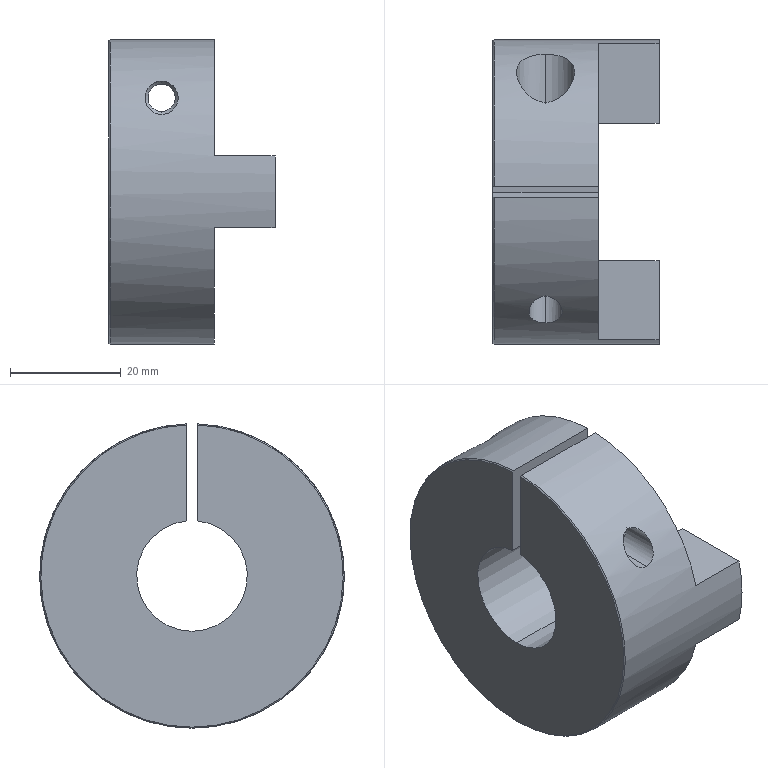Part | STEP file | 0229_Z_MFJC55-20-22_2 | 1 solid | 31 faces | box 30 x 55 x 54.982 mm | volume 40722 mm3 | cylinder 14 | plane 11 | cone 6 | commonest cylinder face diameters 6 x4 4.917 x2 10.5 x2 20 x2 28 x2 55 x2